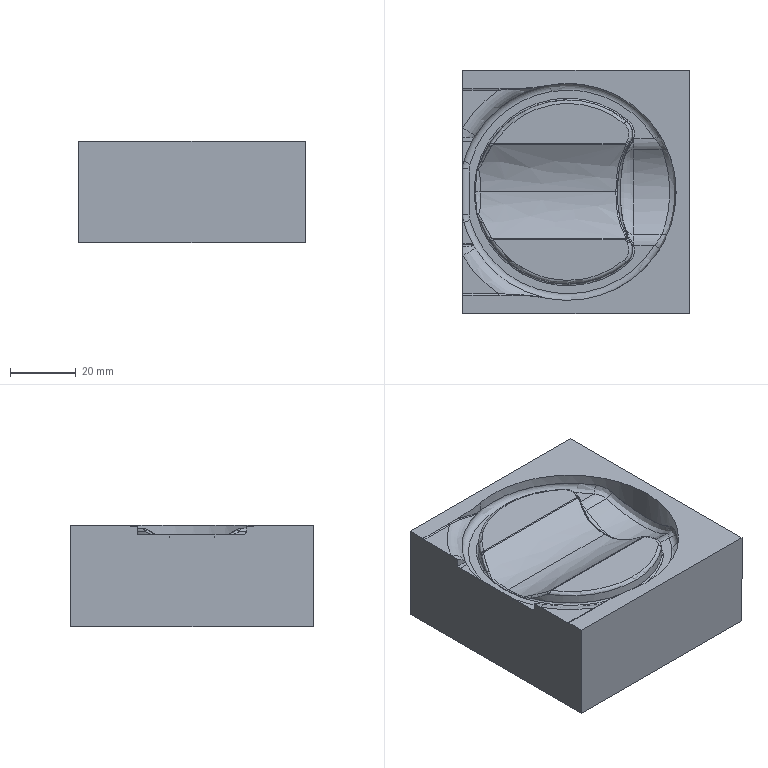NC program | NX | posted with a generic post | part box 69 x 74 x 31.001 mm
Lines 4341 to 5286 of 31411:
(ZLEVEL_PROFILE_COPY , TOOL : D3R0.5)
N8668 M6
N8670 G54
N8672 G17 G0 G90 X10.879 Y6.835 S3000 M3
N8674 G43 Z10.045 H0
N8676 Z0.245
N8678 G94 G1 X0.001 Y6.832 Z-0.04 F2500.
N8680 X11.261 Y6.835
N8682 G3 X16.561 Y6.75 R183.371
N8684 G2 X26.437 Y5.758 R50.425
N8686 G3 X25.948 Y68.154 R-31.734
N8688 G2 X16.456 Y67.239 R49.837
N8690 G3 X10.281 Y67.159 R241.1
N8692 G1 X0. Y67.171
N8694 Y67.112 Z-0.083
N8696 Y67.066 Z-0.125
N8698 G2 X10.037 Y67.051 R2515.475
N8700 X16.412 Y67.135 R232.292
N8702 G3 X23.707 Y67.673 R49.393
N8704 X26.927 Y68.219 R80.541
N8706 G2 X25.947 Y5.954 R-31.63
N8708 G3 X16.646 Y6.865 R51.227
N8710 G2 X11.261 Y6.934 R136.076
N8712 G1 X0.001 Y6.935
N8714 X0. Y6.972 Z-0.168
N8716 Y7.006 Z-0.21
N8718 X0.071 Y7.005
N8720 X0.245 Y6.999
N8722 X1.959 Y7.002
N8724 X10.526 Y7.
N8726 X11.016 Y7.006
N8728 G3 X16.156 Y6.93 R117.76
N8730 G2 X26.192 Y5.971 R51.729
N8732 G3 X27.416 Y68.234 R-31.569
N8734 X25.492 Y67.901 R102.44
N8736 G2 X16.067 Y67.073 R50.738
N8738 G3 X11.016 Y66.994 R117.906
N8740 G1 X9.547 Y66.985
N8742 X0. Y67.002
N8744 Z0.54
N8746 G0 Z10.045
N8748 X6.838 Y61.969
N8750 Z-0.01
N8752 G1 X6.029 Y61.149 Z-0.04
N8754 X4.648 Y59.573 Z-0.095
N8756 X3.362 Y57.918 Z-0.15
N8758 X2.176 Y56.19 Z-0.205
N8760 X1.738 Y55.471 Z-0.227
N8762 X1.601 Y55.223 Z-0.234
N8764 X0.98 Y53.952 Z-0.271
N8766 X0.918 Y53.817 Z-0.275
N8768 X0.713 Y53.579 Z-0.283
N8770 X0.449 Y53.409 Z-0.292
N8772 X0.148 Y53.32 Z-0.3
N8774 X0. Y53.318 Z-0.304
N8776 G3 X0.98 Y53.952 R1.091
N8778 G1 X1.601 Y55.223
N8780 X1.738 Y55.471
N8782 G2 X13.121 Y67.009 R35.454
N8784 X15.667 Y67.026 R73.373
N8786 G3 X24.968 Y67.763 R52.244
N8788 G1 X25.213 Y67.809
N8790 X27.171 Y68.15
N8792 X27.661 Y68.227
N8794 G2 X55.807 Y57.668 R31.529
N8796 X42.837 Y7.393 R31.528
N8798 X31.822 Y5.469 R31.791
N8800 X26.192 Y6.016 R31.756
N8802 G3 X15.667 Y6.969 R52.355
N8804 G2 X13.117 Y6.993 R67.606
N8806 X1.717 Y18.562 R35.454
N8808 G1 X0.94 Y20.085
N8810 G3 X0. Y20.675 R1.082
N8812 G1 Y21.256 Z-0.351
N8814 Y21.646 Z-0.398
N8816 G2 X1.095 Y20.87 R1.155
N8818 G3 X2.204 Y18.559 R12.053
N8820 X13.896 Y6.998 R35.041
N8822 G1 X14.198 Y6.992
N8824 X16.401 Y6.995
N8826 G2 X25.947 Y6.082 R51.929
N8828 G3 X27.661 Y68.206 R-31.505
N8830 X25.703 Y67.872 R62.756
N8832 G2 X16.401 Y67.007 R51.492
N8834 G1 X16.156 Y67.006
N8836 X13.896 Y67.002
N8838 G3 X2.07 Y55.223 R35.041
N8840 X1.068 Y53.099 R14.802
N8842 G2 X0. Y52.358 R1.147
N8844 G1 Y52.288 Z-0.421
N8846 Y52.246 Z-0.444
N8848 Y52.208 Z-0.468
N8850 Y52.187 Z-0.491
N8852 G3 X1.38 Y53.119 R1.486
N8854 G2 X2.337 Y55.061 R14.259
N8856 X14.504 Y67. R34.729
N8858 G1 X16.292
N8860 G3 X26.038 Y67.931 R51.5
N8862 G2 X26.038 Y6.069 R-31.5
N8864 G3 X16.292 Y7. R51.5
N8866 G1 X14.504
N8868 G2 X2.337 Y18.939 R34.729
N8870 X1.388 Y20.876 R13.91
N8872 G3 X0.432 Y21.745 R1.467
N8874 G1 X0.355 Y21.767
N8876 G3 X0. Y21.818 R1.309
N8878 G1 Y21.866 Z-0.538
N8880 Y21.909 Z-0.585
N8882 G2 X0.49 Y21.827 R1.423
N8884 X1.598 Y20.986 R1.646
N8886 G1 X1.714 Y20.728
N8888 X1.811 Y20.497
N8890 X2.448 Y19.274
N8892 X2.559 Y19.074
N8894 G3 X15.026 Y7. R34.469
N8896 G1 X16.292
N8898 G2 X26.038 Y6.069 R51.5
N8900 G3 X26.038 Y67.931 R-31.5
N8902 G2 X16.292 Y67. R51.5
N8904 G1 X15.026
N8906 G3 X2.591 Y54.978 R34.469
N8908 X1.599 Y53.022 R15.137
N8910 G2 X0.49 Y52.171 R1.682
N8912 X0. Y52.09 R1.425
N8914 G1 Y52.064 Z-0.632
N8916 Y52.044 Z-0.679
N8918 G3 X1.097 Y52.303 R2.719
N8920 X1.851 Y53.076 R1.55
N8922 G1 X1.959 Y53.318
N8924 X2.71 Y54.734
N8926 X2.759 Y54.821
N8928 G2 X15.489 Y67. R34.243
N8930 G1 X16.292
N8932 G3 X26.038 Y67.931 R51.5
N8934 G2 X26.038 Y6.069 R-31.5
N8936 G3 X16.292 Y7. R51.5
N8938 G1 X15.489
N8940 G2 X2.751 Y19.192 R34.243
N8942 X1.799 Y21.037 R17.135
N8944 G3 X1.423 Y21.5 R1.132
N8946 X0.245 Y21.937 R2.382
N8948 G1 X0.001 Y21.96
N8950 X0. Y21.976 Z-0.726
N8952 Y21.985 Z-0.773
N8954 X0.082 Y21.983
N8956 X0.245 Y21.973
N8958 G2 X1.307 Y21.712 R3.032
N8960 X1.978 Y21.074 R1.391
N8962 G1 X2.204 Y20.63
N8964 X2.93 Y19.286
N8966 X2.937 Y19.274
N8968 G3 X15.911 Y7. R34.042
N8970 G1 X16.292
N8972 G2 X26.038 Y6.069 R51.5
N8974 G3 X26.038 Y67.931 R-31.5
N8976 G2 X16.292 Y67. R51.5
N8978 G1 X15.911
N8980 G3 X2.923 Y54.703 R34.042
N8982 X2.036 Y53.022 R18.615
N8984 G2 X1.305 Y52.288 R1.509
N8986 X0.001 Y52.014 R3.237
N8988 G1 X0. Y52.005 Z-0.866
N8990 G3 X1.225 Y52.168 R3.767
N8992 X2.204 Y52.973 R1.604
N8994 G1 X2.346 Y53.267
N8996 X3.079 Y54.609
N8998 G2 X16.3 Y67. R33.86
N9000 G3 X26.038 Y67.931 R51.5
N9002 G2 X26.038 Y6.069 R-31.5
N9004 G3 X16.3 Y7. R51.5
N9006 G2 X3.08 Y19.389 R33.86
N9008 G1 X2.344 Y20.741
N9010 X2.239 Y20.966
N9012 G3 X1.277 Y21.815 R1.607
N9014 X0. Y21.996 R3.786
N9016 G1 Y22. Z-0.96
N9018 X0.266
N9020 G2 X1.469 Y21.812 R3.449
N9022 X2.403 Y20.986 R1.561
N9024 G3 X3.218 Y19.476 R19.06
N9026 X16.657 Y6.999 R33.697
N9028 G2 X26.038 Y6.069 R51.5
N9030 G3 X26.038 Y67.931 R-31.5
N9032 G2 X16.657 Y67.001 R51.5
N9034 G3 X3.218 Y54.524 R33.697
N9036 G1 X2.524 Y53.267
N9038 X2.404 Y53.022
N9040 G2 X1.515 Y52.204 R1.574
N9042 X0.492 Y52.007 R3.279
N9044 G1 X0.265 Y52.
N9046 X0.
N9048 Z-1.06
N9050 X0.543
N9052 G3 X1.777 Y52.232 R3.009
N9054 X2.522 Y52.904 R1.513
N9056 G1 X3.252 Y54.245
N9058 X3.363 Y54.436
N9060 G2 X17.04 Y67.005 R33.528
N9062 G3 X26.038 Y67.931 R51.5
N9064 G2 X26.038 Y6.069 R-31.5
N9066 G3 X17.04 Y6.995 R51.5
N9068 G2 X3.363 Y19.564 R33.528
N9070 G1 X3.183 Y19.88
N9072 X2.527 Y21.093
N9074 G3 X1.774 Y21.77 R1.51
N9076 X0.545 Y22. R3.055
N9078 G1 X0.
N9080 Z-1.16
N9082 X0.785
N9084 G2 X2.018 Y21.741 R2.766
N9086 X2.721 Y21.048 R1.475
N9088 G1 X2.869 Y20.741
N9090 X3.493 Y19.643
N9092 G3 X17.399 Y6.988 R33.375
N9094 G2 X26.038 Y6.069 R51.5
N9096 G3 X26.038 Y67.931 R-31.5
N9098 G2 X17.399 Y67.012 R51.5
N9100 G3 X3.493 Y54.357 R33.375
N9102 G1 X3.429 Y54.245
N9104 X2.661 Y52.857
N9106 G2 X2.046 Y52.275 R1.4
N9108 X0.782 Y52. R2.758
N9110 G1 X0.
N9112 Z-0.41
N9114 G0 Z10.045
N9116 X17.708 Y23.823
N9118 Z-0.76
N9120 G1 X29.165 Z-1.06
N9122 X49.452
N9124 G2 X51.033 Y22.698 R1.739
N9126 X51.649 Y17.04 R5.734
N9128 X50.142 Y15.058 R5.972
N9130 X7.975 Y21.724 R28.471
N9132 X8.883 Y23.75 R1.33
N9134 G1 X9.302 Y23.818
N9136 X9.391 Y23.823
N9138 X29.165
N9140 Y23.919 Z-1.11
N9142 Y23.998 Z-1.16
N9144 X8.999 Y23.995
N9146 G3 X7.729 Y21.723 R1.491
N9148 G1 X7.791 Y21.622
N9150 G3 X50.277 Y14.898 R28.68
N9152 X51.777 Y21.799 R5.716
N9154 X50.92 Y23.292 R12.461
N9156 X49.589 Y24.002 R1.601
N9158 G1 X29.165 Y23.998
N9160 Y24.085 Z-1.21
N9162 Y24.166 Z-1.26
N9164 X49.624 Y24.167
N9166 G2 X51.014 Y23.426 R1.676
N9168 X52.093 Y21.475 R12.777
N9170 X50.372 Y14.78 R5.938
N9172 X7.615 Y21.617 R28.832
N9174 X7.411 Y23.187 R1.824
N9176 X8.766 Y24.165 R1.428
N9178 G1 X29.165 Y24.166
N9180 Z-0.51
N9182 G0 Z10.045
N9184 X40.817 Y50.177
N9186 Z-0.76
N9188 G1 X29.361 Z-1.06
N9190 X9.249
N9192 G2 X7.868 Y51.066 R1.518
N9194 X7.948 Y52.235 R1.231
N9196 X50.142 Y58.942 R28.471
N9198 X51.32 Y51.799 R5.531
N9200 G1 X50.67 Y50.737
N9202 X50.596 Y50.659
N9204 G2 X49.472 Y50.177 R1.552
N9206 G1 X29.361
N9208 Y50.08 Z-1.11
N9210 X29.36 Y50.001 Z-1.16
N9212 X49.598 Y49.998
N9214 G3 X50.848 Y50.619 R1.569
N9216 G1 X51.002 Y50.821
N9218 X51.583 Y51.825
N9220 G3 X50.276 Y59.103 R5.724
N9222 X7.788 Y52.374 R28.68
N9224 G1 X7.732 Y52.288
N9226 G3 X9.058 Y50.005 R1.499
N9228 G1 X29.36 Y50.001
N9230 Y49.915 Z-1.21
N9232 Y49.834 Z-1.26
N9234 X8.813 Y49.835
N9236 G2 X7.324 Y51.555 R1.512
N9238 X7.615 Y52.383 R2.184
N9240 X50.372 Y59.22 R28.832
N9242 X51.877 Y52.044 R5.929
N9244 G1 X51.16 Y50.796
N9246 X51.058 Y50.633
N9248 G2 X49.62 Y49.833 R1.694
N9250 G1 X29.36 Y49.834
N9252 Z-0.51
N9254 G0 Z10.045
N9256 X7.66 Y14.382
N9258 Z-0.96
N9260 G1 X6.667 Y15.475 Z-0.999
N9262 X5.294 Y17.204 Z-1.056
N9264 X4.039 Y19.021 Z-1.114
N9266 X3.615 Y19.717 Z-1.136
N9268 X2.906 Y20.986 Z-1.174
N9270 X2.758 Y21.256 Z-1.182
N9272 X2.485 Y21.556 Z-1.192
N9274 X2.145 Y21.777 Z-1.203
N9276 X1.751 Y21.917 Z-1.214
N9278 X1.24 Y22.002 Z-1.228
N9280 X1.001 Y22. Z-1.234
N9282 X0. Z-1.26
N9284 X1.001
N9286 G2 X1.977 Y21.837 R2.859
N9288 X2.844 Y21.099 R1.593
N9290 G1 X2.906 Y20.986
N9292 X3.615 Y19.717
N9294 G3 X17.745 Y6.979 R33.233
N9296 G2 X26.038 Y6.069 R51.5
N9298 G3 X26.038 Y67.931 R-31.5
N9300 G2 X17.745 Y67.021 R51.5
N9302 G3 X3.672 Y54.377 R33.233
N9304 G1 X3.612 Y54.285
N9306 X2.837 Y52.892
N9308 G2 X1.979 Y52.166 R1.59
N9310 X0.996 Y52. R2.885
N9312 G1 X0.
N9314 Z-1.36
N9316 X1.193
N9318 G3 X2.174 Y52.179 R2.635
N9320 X2.989 Y52.9 R1.573
N9322 G1 X3.054 Y53.022
N9324 X3.603 Y54.
N9326 X3.728 Y54.213
N9328 G2 X18.082 Y67.031 R33.1
N9330 G3 X26.038 Y67.931 R51.5
N9332 G2 X26.038 Y6.069 R-31.5
N9334 G3 X18.082 Y6.969 R51.5
N9336 G2 X3.728 Y19.787 R33.1
N9338 G1 X3.672 Y19.882
N9340 X3.051 Y20.986
N9342 X2.99 Y21.099
N9344 G3 X2.159 Y21.828 R1.563
N9346 X1.197 Y22. R2.706
N9348 G1 X0.
N9350 Z-0.61
N9352 G0 Z10.045
N9354 X17.674 Y24.331
N9356 Z-1.06
N9358 G1 X29.131 Y24.332 Z-1.36
N9360 X49.573
N9362 G2 X51.172 Y23.419 R1.856
N9364 G1 X51.894 Y22.194
N9366 G2 X50.449 Y14.687 R6.036
N9368 X7.485 Y21.598 R28.952
N9370 X7.145 Y22.758 R2.305
N9372 X8.688 Y24.331 R1.543
N9374 G1 X29.131 Y24.332
N9376 Y24.414 Z-1.41
N9378 Y24.496 Z-1.46
N9380 X8.568 Y24.495
N9382 G3 X7.036 Y23.187 R1.539
N9384 X7.353 Y21.623 R2.214
N9386 X50.511 Y14.612 R29.05
N9388 G1 X50.79 Y14.872
N9390 G3 X51.994 Y22.209 R6.105
N9392 G1 X51.863 Y22.453
N9394 X51.279 Y23.431
N9396 X51.16 Y23.612
N9398 G3 X49.446 Y24.497 R2.002
N9400 G1 X29.131 Y24.496
N9402 Z-0.71
N9404 G0 Z10.045
N9406 X40.588 Y49.668
N9408 Z-1.06
N9410 G1 X29.131 Z-1.36
N9412 X8.689 Y49.669
N9414 G2 X7.145 Y51.244 R1.544
N9416 X7.486 Y52.404 R2.306
N9418 X50.449 Y59.313 R28.952
N9420 X51.753 Y51.555 R6.041
N9422 G1 X51.649 Y51.387
N9424 X51.607 Y51.31
N9426 X51.166 Y50.572
N9428 G2 X49.574 Y49.668 R1.855
N9430 G1 X29.131
N9432 Y49.586 Z-1.41
N9434 Y49.504 Z-1.46
N9436 X49.507 Y49.503
N9438 G3 X51.212 Y50.472 R1.984
N9440 G1 X51.274 Y50.576
N9442 G3 X51.99 Y51.786 R17.302
N9444 X51.284 Y58.602 R6.091
N9446 X50.511 Y59.388 R7.291
N9448 X7.353 Y52.377 R29.05
N9450 X7.034 Y50.821 R2.236
N9452 X8.568 Y49.505 R1.54
N9454 G1 X29.131 Y49.504
N9456 Z-0.71
N9458 G0 Z10.045
N9460 X7.79 Y14.627
N9462 Z-1.16
N9464 G1 X6.965 Y15.525 Z-1.192
N9466 X5.549 Y17.295 Z-1.251
N9468 X4.258 Y19.158 Z-1.311
N9470 X3.836 Y19.852 Z-1.332
N9472 X3.192 Y20.986 Z-1.366
N9474 X3.183 Y21.006 Z-1.367
N9476 X3.106 Y21.169 Z-1.371
N9478 X2.817 Y21.521 Z-1.383
N9480 X2.443 Y21.779 Z-1.395
N9482 X2.274 Y21.842 Z-1.4
N9484 X2.058 Y21.92 Z-1.406
N9486 X1.607 Y22. Z-1.418
N9488 X1.378 Z-1.424
N9490 X0. Z-1.46
N9492 X1.378
N9494 G2 X2.274 Y21.842 R2.633
N9496 X3.183 Y21.006 R1.629
N9498 G1 X3.192 Y20.986
N9500 X3.836 Y19.852
N9502 G3 X18.411 Y6.956 R32.974
N9504 G2 X26.038 Y6.069 R51.5
N9506 G3 X26.038 Y67.931 R-31.5
N9508 G2 X18.411 Y67.044 R51.5
N9510 G3 X3.836 Y54.148 R32.974
N9512 G1 X3.196 Y53.022
N9514 X3.136 Y52.91
N9516 G2 X2.28 Y52.162 R1.587
N9518 X1.374 Y52. R2.651
N9520 G1 X0.
N9522 Z-1.56
N9524 X1.541
N9526 G3 X2.473 Y52.181 R2.45
N9528 X3.21 Y52.824 R1.506
N9530 G1 X3.937 Y54.087
N9532 G2 X18.732 Y67.058 R32.856
N9534 G3 X26.038 Y67.931 R51.5
N9536 G2 X26.038 Y6.069 R-31.5
N9538 G3 X18.732 Y6.942 R51.5
N9540 G2 X3.937 Y19.913 R32.856
N9542 G1 X3.32 Y20.986
N9544 X3.255 Y21.108
N9546 G3 X2.519 Y21.797 R1.554
N9548 X1.545 Y22. R2.317
N9550 G1 X0.
N9552 Z-0.81
N9554 G0 Z10.045
N9556 X17.467 Y24.662
N9558 Z-1.26
N9560 G1 X28.923 Z-1.56
N9562 X49.373
N9564 G2 X51.236 Y23.649 R2.218
N9566 X51.956 Y22.453 R21.602
N9568 G1 X52.087 Y22.209
N9570 G2 X50.564 Y14.548 R6.206
N9572 X7.246 Y21.64 R29.132
N9574 X6.954 Y23.494 R2.317
N9576 X8.474 Y24.662 R1.573
N9578 G1 X28.923
N9580 Y24.744 Z-1.61
N9582 Y24.827 Z-1.66
N9584 X8.398
N9586 G3 X6.823 Y23.562 R1.612
N9588 X7.158 Y21.65 R2.546
N9590 G1 X7.268 Y21.475
N9592 G3 X50.607 Y14.495 R29.201
N9594 G1 X50.915 Y14.78
N9596 G3 X52.139 Y22.259 R6.258
N9598 X51.238 Y23.765 R18.269
N9600 X49.256 Y24.827 R2.38
N9602 G1 X28.923
N9604 Z-0.91
N9606 G0 Z10.045
N9608 X40.379 Y49.338
N9610 Z-1.26
N9612 G1 X28.922 Z-1.56
N9614 X8.473
N9616 G2 X6.955 Y50.503 R1.572
N9618 X7.246 Y52.36 R2.317
N9620 X50.564 Y59.452 R29.132
N9622 X52.09 Y51.799 R6.206
N9624 G1 X52.072 Y51.765
N9626 G2 X51.236 Y50.35 R19.155
N9628 X49.371 Y49.338 R2.224
N9630 G1 X28.922
N9632 Y49.256 Z-1.61
N9634 Y49.173 Z-1.66
N9636 X49.262
N9638 G3 X51.219 Y50.211 R2.363
N9640 X52.164 Y51.795 R16.025
N9642 X51.186 Y58.944 R6.239
N9644 X50.607 Y59.505 R8.382
N9646 X7.164 Y52.359 R29.201
N9648 X6.844 Y50.351 R2.544
N9650 X8.364 Y49.173 R1.57
N9652 G1 X28.922
N9654 Z-0.91
N9656 G0 Z10.045
N9658 X7.899 Y14.839
N9660 Z-1.36
N9662 G1 X6.902 Y15.954 Z-1.399
N9664 X5.625 Y17.579 Z-1.453
N9666 X4.453 Y19.28 Z-1.507
N9668 X4.032 Y19.972 Z-1.529
N9670 X3.447 Y20.986 Z-1.559
N9672 X3.266 Y21.314 Z-1.569
N9674 X2.927 Y21.65 Z-1.582
N9676 X2.593 Y21.831 Z-1.591
N9678 X2.259 Y21.943 Z-1.601
N9680 X1.911 Y22.002 Z-1.61
N9682 X1.7 Y22. Z-1.615
N9684 X0. Z-1.66
N9686 X1.7
N9688 G2 X2.779 Y21.731 R2.227
N9690 X3.347 Y21.166 R1.425
N9692 G1 X3.447 Y20.986
N9694 X4.032 Y19.972
N9696 G3 X19.049 Y6.926 R32.744
N9698 G2 X26.038 Y6.069 R51.5
N9700 G3 X26.038 Y67.931 R-31.5
N9702 G2 X19.049 Y67.074 R51.5
N9704 G3 X4.032 Y54.028 R32.744
N9706 G1 X4.014 Y54.
N9708 X3.451 Y53.022
N9710 X3.428 Y52.978
N9712 X3.317 Y52.777
N9714 G2 X2.448 Y52.121 R1.646
N9716 X1.697 Y52. R2.534
N9718 G1 X0.
N9720 Z-1.76
N9722 X1.843
N9724 G3 X2.7 Y52.166 R2.367
N9726 X3.451 Y52.813 R1.51
N9728 G1 X4.123 Y53.973
N9730 G2 X19.361 Y67.092 R32.638
N9732 G3 X26.038 Y67.931 R51.5
N9734 G2 X26.038 Y6.069 R-31.5
N9736 G3 X19.361 Y6.908 R51.5
N9738 G2 X4.123 Y20.027 R32.638
N9740 G1 X3.451 Y21.185
N9742 G3 X2.7 Y21.834 R1.524
N9744 X1.846 Y22. R2.305
N9746 G1 X0.
N9748 Z-1.01
N9750 G0 Z10.045
N9752 X17.428 Y24.989
N9754 Z-1.46
N9756 G1 X28.885 Y24.987 Z-1.76
N9758 X49.446 Y24.983
N9760 G2 X51.284 Y23.804 R2.686
N9762 X52.179 Y22.306 R19.901
N9764 X50.96 Y14.747 R6.291
N9766 G1 X50.67 Y14.473
N9768 X50.644 Y14.451
N9770 G2 X7.082 Y21.664 R29.259
N9772 X6.781 Y23.92 R2.718
N9774 X8.323 Y24.991 R1.567
N9776 G1 X28.885 Y24.987
N9778 Y25.074 Z-1.81
N9780 Y25.156 Z-1.86
N9782 X8.18
N9784 G3 X6.61 Y23.846 R1.597
N9786 X6.993 Y21.718 R3.08
N9788 X50.675 Y14.414 R29.307
N9790 X52.759 Y20.986 R6.393
N9792 X52.162 Y22.443 R6.655
N9794 X51.279 Y23.901 R22.919
N9796 G1 X51.266 Y23.92
N9798 G3 X50.359 Y24.778 R3.439
N9800 X49.075 Y25.156 R2.37
N9802 G1 X28.885
N9804 Z-1.11
N9806 G0 Z10.045
N9808 X40.341 Y49.016
N9810 Z-1.46
N9812 G1 X28.885 Y49.013 Z-1.76
N9814 X8.323 Y49.008
N9816 G2 X6.778 Y50.087 R1.568
N9818 X7.069 Y52.314 R2.73
N9820 X50.644 Y59.549 R29.259
N9822 X51.405 Y58.795 R10.522
N9824 X51.96 Y51.31 R6.328
N9826 X51.207 Y50.087 R13.127
N9828 X49.446 Y49.018 R2.666
N9830 G1 X28.885 Y49.013
N9832 Y48.926 Z-1.81
N9834 Y48.844 Z-1.86
N9836 X49.144
N9838 G3 X50.185 Y49.115 R2.131
N9840 X51.361 Y50.221 R3.332
N9842 X52.16 Y51.555 R24.616
N9844 X52.355 Y57.424 R6.365
N9846 X50.675 Y59.586 R6.543
N9848 X6.997 Y52.289 R29.307
N9850 X6.61 Y50.153 R3.074
N9852 X8.181 Y48.844 R1.598
N9854 G1 X28.885
N9856 Z-1.11
N9858 G0 Z10.045
N9860 X8.003 Y15.037
N9862 Z-1.56
N9864 G1 X7.145 Y15.986 Z-1.594
N9866 X5.831 Y17.647 Z-1.649
N9868 X4.628 Y19.39 Z-1.704
N9870 X4.209 Y20.079 Z-1.726
N9872 X3.479 Y21.341 Z-1.764
N9874 X3.172 Y21.645 Z-1.775
N9876 X2.846 Y21.83 Z-1.785
N9878 X2.523 Y21.942 Z-1.794
N9880 X2.187 Y22.001 Z-1.803
N9882 X1.982 Y22. Z-1.808
N9884 X0. Z-1.86
N9886 X1.982
N9888 G2 X3.024 Y21.729 R2.089
N9890 X3.564 Y21.193 R1.448
N9892 G1 X4.209 Y20.079
N9894 G3 X19.671 Y6.889 R32.537
N9896 G2 X26.038 Y6.069 R51.5
N9898 G3 X26.038 Y67.931 R-31.5
N9900 G2 X19.671 Y67.111 R51.5
N9902 G3 X4.209 Y53.921 R32.537
N9904 G1 X3.59 Y52.847
N9906 G2 X2.708 Y52.123 R1.617
N9908 X1.98 Y52. R2.317
N9910 G1 X0.
N9912 Z-1.96
N9914 X2.111
N9916 G3 X2.876 Y52.141 R2.264
N9918 X3.694 Y52.834 R1.577
N9920 G1 X4.29 Y53.871
N9922 G2 X19.978 Y67.132 R32.442
N9924 G3 X26.038 Y67.931 R51.5
N9926 G2 X26.038 Y6.069 R-31.5
N9928 G3 X19.978 Y6.868 R51.5
N9930 G2 X4.29 Y20.129 R32.442
N9932 G1 X4.215 Y20.252
N9934 X3.672 Y21.197
N9936 G3 X3.154 Y21.72 R1.54
N9938 X2.11 Y22. R2.033
N9940 G1 X0.
N9942 Z-1.21
N9944 G0 Z10.045
N9946 X40.023 Y48.679
N9948 Z-1.66
N9950 G1 X28.567 Z-1.96
N9952 X8.078
N9954 G2 X6.495 Y50.087 R1.602
N9956 X6.944 Y52.277 R3.345
N9958 X50.7 Y59.617 R29.346
N9960 X51.588 Y58.703 R7.264
N9962 X52.451 Y52.053 R6.369
N9964 X51.924 Y51.066 R8.654
N9966 X51.321 Y50.087 R17.898
N9968 X50.161 Y48.988 R3.787
N9970 X49.055 Y48.679 R2.13
N9972 G1 X28.567
N9974 Y48.596 Z-2.01
N9976 Y48.514 Z-2.06
N9978 X48.957
N9980 G3 X50.153 Y48.869 R2.105
N9982 X51.312 Y50.025 R4.235
N9984 X52.24 Y51.555 R19.132
N9986 X52.31 Y57.668 R6.415
N9988 X51.16 Y59.237 R6.686
N9990 G1 X50.72 Y59.641
N9992 G3 X6.873 Y52.221 R29.378
N9994 X6.37 Y50.087 R3.738
N9996 X8.078 Y48.514 R1.662
N9998 G1 X28.567
N10000 Z-1.31
N10002 G0 Z10.045
N10004 X17.076 Y25.32
N10006 Z-1.66
N10008 G1 X28.533 Y25.321 Z-1.96
N10010 X48.987
N10012 G2 X50.208 Y24.977 R2.338
N10014 X51.314 Y23.92 R3.616
N10016 X52.264 Y22.33 R19.121
N10018 X51.253 Y14.91 R6.396
N10020 G1 X51.16 Y14.812
N10022 X50.7 Y14.383
N10024 G2 X6.928 Y21.749 R29.346
N10026 X6.497 Y23.92 R3.344
N10028 X8.078 Y25.32 R1.6
N10030 G1 X28.533 Y25.321
N10032 Y25.404 Z-2.01
N10034 Y25.486 Z-2.06
N10036 X7.926
N10038 G3 X7.099 Y25.218 R1.408
N10040 X6.365 Y23.852 R1.783
N10042 X6.87 Y21.784 R3.817
N10044 X50.72 Y14.359 R29.378
N10046 G1 X51.19 Y14.793
N10048 X51.262 Y14.872
N10050 X51.405 Y15.025
N10052 G3 X52.923 Y18.051 R6.426
N10054 X52.235 Y22.453 R6.436
N10056 X51.351 Y23.92 R20.72
N10058 X50.344 Y25.003 R4.602
N10060 X48.933 Y25.486 R2.301
N10062 G1 X28.533
N10064 Z-1.31
N10066 G0 Z10.045
N10068 X8.095 Y15.214
N10070 Z-1.76
N10072 G1 X7.373 Y16.007 Z-1.788
N10074 X6.021 Y17.705 Z-1.845
N10076 X4.786 Y19.489 Z-1.902
N10078 X4.368 Y20.176 Z-1.923
N10080 X3.757 Y21.23 Z-1.955
N10082 X3.664 Y21.378 Z-1.959
N10084 X3.337 Y21.683 Z-1.971
N10086 X3.183 Y21.765 Z-1.976
N10088 X3.004 Y21.859 Z-1.981
N10090 X2.724 Y21.95 Z-1.989
N10092 X2.434 Y22. Z-1.996
N10094 X2.232 Z-2.002
N10096 X0. Z-2.06
N10098 X2.232
N10100 G2 X3.183 Y21.765 R2.033
N10102 X3.757 Y21.23 R1.516
N10104 G1 X4.368 Y20.176
N10106 G3 X20.285 Y6.845 R32.351
N10108 G2 X26.038 Y6.069 R51.5
N10110 G3 X26.038 Y67.931 R-31.5
N10112 G2 X20.285 Y67.155 R51.5
N10114 G3 X4.368 Y53.824 R32.351
N10116 G1 X3.795 Y52.835
N10118 G2 X2.927 Y52.12 R1.613
N10120 X2.234 Y52. R2.175
N10122 G1 X0.
N10124 Z-2.16
N10126 X2.35
N10128 G3 X3.152 Y52.166 R2.102
N10130 X3.917 Y52.874 R1.589
N10132 G1 X4.407 Y53.721
N10134 X4.442 Y53.779
N10136 G2 X20.591 Y67.18 R32.264
N10138 G3 X26.038 Y67.931 R51.5
N10140 G2 X26.038 Y6.069 R-31.5
N10142 G3 X20.591 Y6.82 R51.5
N10144 G2 X4.445 Y20.216 R32.264
N10146 G1 X3.855 Y21.23
N10148 G3 X3.366 Y21.72 R1.442
N10150 X2.347 Y22. R1.932
N10152 G1 X0.
N10154 Z-1.41
N10156 G0 Z10.045
N10158 X16.899 Y25.65
N10160 Z-1.86
N10162 G1 X28.356 Z-2.16
N10164 X48.881 Y25.651
N10166 G2 X50.133 Y25.253 R2.172
N10168 X51.214 Y24.165 R4.418
N10170 X52.295 Y22.393 R19.903
N10172 X52.345 Y16.341 R6.459
N10174 X51.001 Y14.585 R6.391
N10176 G1 X50.735 Y14.341
N10178 G2 X6.819 Y21.821 R29.402
N10180 X6.259 Y23.867 R4.207
N10182 X6.725 Y25.143 R1.917
N10184 X7.831 Y25.65 R1.461
N10186 G1 X28.356
N10188 Y25.734 Z-2.21
N10190 Y25.816 Z-2.26
N10192 X7.781
N10194 G3 X6.337 Y24.844 R1.56
N10196 X6.178 Y23.676 R2.369
N10198 X6.775 Y21.862 R4.574
N10200 X50.746 Y14.328 R29.419
N10202 G1 X51.015 Y14.575
N10204 G3 X52.342 Y22.338 R6.452
N10206 X51.066 Y24.41 R18.727
N10208 X49.952 Y25.482 R4.153
N10210 X48.831 Y25.816 R2.049
N10212 G1 X28.356
N10214 Z-1.51
N10216 G0 Z10.045
N10218 X39.881 Y48.35
N10220 Z-1.86
N10222 G1 X28.424 Z-2.16
N10224 X7.892
N10226 G2 X6.329 Y49.616 R1.598
N10228 X6.326 Y50.86 R3.026
N10230 X6.82 Y52.181 R4.603
N10232 X50.735 Y59.659 R29.402
N10234 X51.708 Y58.647 R7.147
N10236 X52.269 Y51.555 R6.453
N10238 X51.22 Y49.843 R21.314
N10240 X50.181 Y48.78 R4.465
N10242 X48.957 Y48.349 R2.131
N10244 G1 X28.424 Y48.35
N10246 Y48.267 Z-2.21
N10248 Y48.184 Z-2.26
N10250 X48.839
N10252 G3 X49.928 Y48.503 R2.019
N10254 X51.053 Y49.571 R4.103
N10256 X51.989 Y51.029 R17.178
N10258 G1 X52.289 Y51.555
N10260 G3 X52.873 Y56.352 R6.499
N10262 X50.746 Y59.672 R6.604
N10264 X6.776 Y52.139 R29.419
N10266 X6.398 Y51.31 R5.41
N10268 G1 X6.365 Y51.217
N10270 G3 X6.206 Y49.598 R3.322
N10272 X7.834 Y48.184 R1.615
N10274 G1 X28.424
N10276 Z-1.51
N10278 G0 Z10.045
N10280 X8.174 Y15.38
N10282 Z-1.96
N10284 G1 X7.587 Y16.016 Z-1.983
N10286 X6.197 Y17.751 Z-2.041
N10288 X4.93 Y19.579 Z-2.099
N10290 X4.512 Y20.264 Z-2.12
N10292 X4.407 Y20.44 Z-2.125
N10294 X3.947 Y21.23 Z-2.149
N10296 X3.86 Y21.379 Z-2.154
N10298 X3.627 Y21.624 Z-2.163
N10300 X3.344 Y21.811 Z-2.172
N10302 X3.183 Y21.87 Z-2.176
N10304 X2.987 Y21.941 Z-2.182
N10306 X2.666 Y21.999 Z-2.19
N10308 X2.457 Y22. Z-2.196
N10310 X0. Z-2.26
N10312 X2.457
N10314 G2 X3.183 Y21.87 R2.164
N10316 X3.947 Y21.23 R1.478
N10318 G1 X4.407 Y20.44
N10320 X4.512 Y20.264
N10322 G3 X20.899 Y6.794 R32.182
N10324 G2 X26.038 Y6.069 R51.5
N10326 G3 X26.038 Y67.931 R-31.5
N10328 G2 X20.899 Y67.207 R51.5
N10330 G3 X4.512 Y53.736 R32.182
N10332 G1 X3.984 Y52.829
N10334 G2 X2.933 Y52.059 R1.629
N10336 X2.46 Y52. R2.504
N10338 G1 X0.
N10340 Z-2.36
N10342 X2.564
N10344 G3 X4.041 Y52.777 R1.702
N10346 G1 X4.162 Y52.98
N10348 X4.58 Y53.695
N10350 G2 X21.21 Y67.235 R32.103
N10352 G3 X26.038 Y67.931 R51.5
N10354 G2 X26.038 Y6.069 R-31.5
N10356 G3 X21.21 Y6.765 R51.5
N10358 G2 X4.58 Y20.305 R32.103
N10360 G1 X4.04 Y21.23
N10362 G3 X3.019 Y21.963 R1.469
N10364 X2.612 Y22. R2.263
N10366 G1 X0.
N10368 Z-1.61
N10370 G0 Z10.045
N10372 X16.766 Y25.981
N10374 Z-2.06
N10376 G1 X28.223 Z-2.36
N10378 X48.712
N10380 G2 X49.936 Y25.607 R2.077
N10382 X51.099 Y24.41 R4.601
N10384 G1 X51.16 Y24.321
N10386 G2 X52.296 Y22.453 R24.503
N10388 X50.826 Y14.383 R6.491
N10390 G1 X50.79 Y14.355
N10392 X50.753 Y14.32
N10394 G2 X6.737 Y21.905 R29.429
N10396 X6.267 Y22.942 R5.993
N10398 X6.093 Y24.503 R3.692
N10400 X7.733 Y25.981 R1.649
N10402 G1 X28.223
N10404 Y26.064 Z-2.41
N10406 Y26.145 Z-2.46
N10408 X7.608
N10410 G3 X6.091 Y25.014 R1.583
N10412 X6.027 Y23.676 R2.791
N10414 X6.643 Y22.054 R5.135
N10416 X50.76 Y14.319 R29.434
N10418 X52.167 Y22.698 R6.503
N10420 G1 X52.139 Y22.743
N10422 G3 X50.956 Y24.654 R21.963
N10424 X49.936 Y25.718 R4.527
N10426 X48.712 Y26.145 R2.105
N10428 G1 X28.223
N10430 Z-1.71
N10432 G0 Z10.045
N10434 X39.68 Y48.019
N10436 Z-2.06
N10438 G1 X28.224 Z-2.36
N10440 X7.735
N10442 G2 X6.091 Y49.509 R1.652
N10444 X6.269 Y51.066 R3.717
N10446 X6.738 Y52.095 R5.819
N10448 X50.753 Y59.68 R29.429
N10450 X53.09 Y54.245 R6.52
N10452 X52.163 Y51.31 R6.619
N10454 G1 X52.139 Y51.271
N10456 G2 X51.104 Y49.598 R21.546
N10458 X49.936 Y48.393 R4.625
N10460 X48.712 Y48.019 R2.054
N10462 G1 X28.224
N10464 Y47.937 Z-2.41
N10466 Y47.855 Z-2.46
N10468 X48.712
N10470 G3 X49.936 Y48.282 R2.101
N10472 X50.961 Y49.354 R4.532
N10474 X52.139 Y51.257 R23.428
N10476 G1 X52.172 Y51.31
N10478 G3 X53.111 Y54.489 R6.616
N10480 X50.76 Y59.681 R6.52
N10482 X6.643 Y51.946 R29.434
N10484 X6.029 Y50.332 R5.115
N10486 X6.098 Y48.965 R2.757
N10488 X7.606 Y47.855 R1.579
N10490 G1 X28.224
N10492 Z-1.71
N10494 G0 Z10.045
N10496 X8.226 Y15.548
N10498 Z-2.16
N10500 G1 X7.497 Y16.36 Z-2.189
N10502 X6.225 Y17.971 Z-2.242
N10504 X5.06 Y19.66 Z-2.296
N10506 X4.644 Y20.344 Z-2.317
N10508 X4. Y21.449 Z-2.35
N10510 X3.723 Y21.728 Z-2.361
N10512 X3.382 Y21.924 Z-2.371
N10514 X3.001 Y22.023 Z-2.381
N10516 X0.001 Z-2.46
N10518 X2.83
N10520 G2 X4.086 Y21.301 R1.454
N10522 G1 X4.644 Y20.344
N10524 G3 X21.525 Y6.733 R32.028
N10526 G2 X26.038 Y6.069 R51.5
N10528 G3 X26.038 Y67.931 R-31.5
N10530 G2 X21.525 Y67.267 R51.5
N10532 G3 X4.644 Y53.656 R32.028
N10534 G1 X4.554 Y53.511
N10536 X4.162 Y52.835
N10538 G2 X3.183 Y52.075 R1.577
N10540 X2.663 Y52. R2.163
N10542 G1 X0.
N10544 Z-2.56
N10546 X2.758
N10548 G3 X3.428 Y52.127 R1.888
N10550 X4.208 Y52.777 R1.569
N10552 G1 X4.705 Y53.619